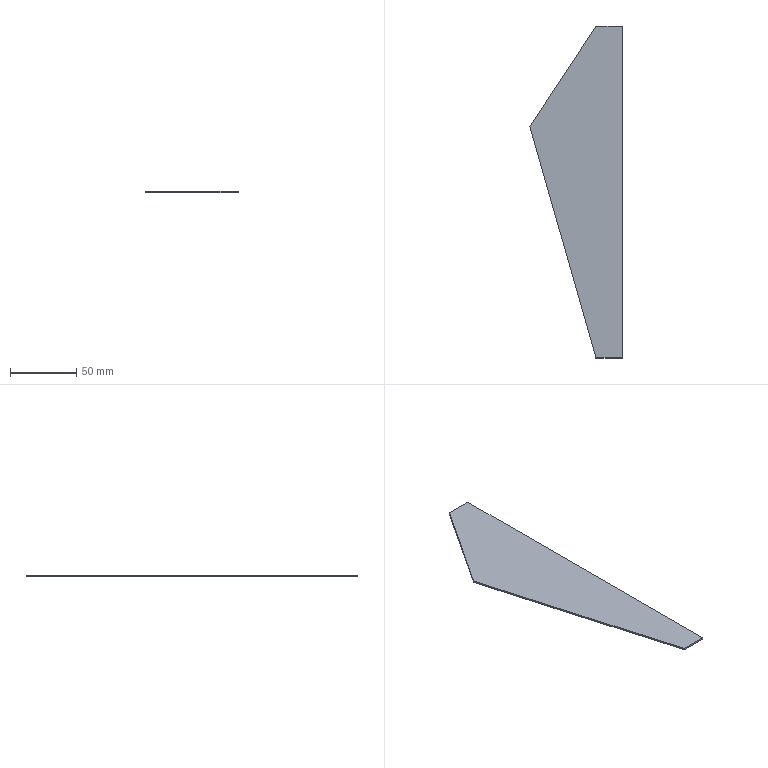Part | SolidWorks | features FlatPattern 1, SMBaseFlange 1, SheetMetal 1 | 1 solid | 7 faces | box 69.783 x 250.8 x 1.2 mm | volume 13490 mm3 | plane 7
STEP:
#1=CARTESIAN_POINT('',(-61.583,173.767,0.));
#2=VERTEX_POINT('',#1);
#3=CARTESIAN_POINT('',(-11.649,-1.,0.));
#4=VERTEX_POINT('',#3);
#5=CARTESIAN_POINT('',(-61.583,173.767,0.));
#6=DIRECTION('',(0.2747,-0.9615,0.));
#7=VECTOR('',#6,1000.);
#8=LINE('',#5,#7);
#9=EDGE_CURVE('',#2,#4,#8,.T.);
#10=ORIENTED_EDGE('',*,*,#9,.F.);
#11=CARTESIAN_POINT('',(-61.583,173.767,-1.2));
#12=VERTEX_POINT('',#11);
#13=CARTESIAN_POINT('',(-61.583,173.767,-1.2));
#14=DIRECTION('',(0.,0.,1.));
#15=VECTOR('',#14,1000.);
#16=LINE('',#13,#15);
#17=EDGE_CURVE('',#12,#2,#16,.T.);
#18=ORIENTED_EDGE('',*,*,#17,.F.);
#19=CARTESIAN_POINT('',(-11.649,-1.,-1.2));
#20=VERTEX_POINT('',#19);
#21=CARTESIAN_POINT('',(-61.583,173.767,-1.2));
#22=DIRECTION('',(0.2747,-0.9615,0.));
#23=VECTOR('',#22,1000.);
#24=LINE('',#21,#23);
#25=EDGE_CURVE('',#12,#20,#24,.T.);
#26=ORIENTED_EDGE('',*,*,#25,.T.);
#27=CARTESIAN_POINT('',(-11.649,-1.,-1.2));
#28=DIRECTION('',(0.,0.,1.));
#29=VECTOR('',#28,1000.);
#30=LINE('',#27,#29);
#31=EDGE_CURVE('',#20,#4,#30,.T.);
#32=ORIENTED_EDGE('',*,*,#31,.T.);
#33=EDGE_LOOP('',(#10,#18,#26,#32));
#34=FACE_OUTER_BOUND('',#33,.T.);
#35=CARTESIAN_POINT('',(-61.583,173.767,-1.2));
#36=DIRECTION('',(-0.9615,-0.2747,0.));
#37=DIRECTION('',(0.2747,-0.9615,0.));
#38=AXIS2_PLACEMENT_3D('',#35,#36,#37);
#39=PLANE('',#38);
#40=ADVANCED_FACE('',(#34),#39,.T.);
#41=CARTESIAN_POINT('',(-11.692,249.8,0.));
#42=VERTEX_POINT('',#41);
#43=CARTESIAN_POINT('',(-61.583,173.767,0.));
#44=DIRECTION('',(-0.5486,-0.8361,0.));
#45=VECTOR('',#44,1000.);
#46=LINE('',#43,#45);
#47=EDGE_CURVE('',#42,#2,#46,.T.);
#48=ORIENTED_EDGE('',*,*,#47,.F.);
#49=CARTESIAN_POINT('',(-11.692,249.8,-1.2));
#50=VERTEX_POINT('',#49);
#51=CARTESIAN_POINT('',(-11.692,249.8,-1.2));
#52=DIRECTION('',(0.,0.,1.));
#53=VECTOR('',#52,1000.);
#54=LINE('',#51,#53);
#55=EDGE_CURVE('',#50,#42,#54,.T.);
#56=ORIENTED_EDGE('',*,*,#55,.F.);
#57=CARTESIAN_POINT('',(-61.583,173.767,-1.2));
#58=DIRECTION('',(-0.5486,-0.8361,0.));
#59=VECTOR('',#58,1000.);
#60=LINE('',#57,#59);
#61=EDGE_CURVE('',#50,#12,#60,.T.);
#62=ORIENTED_EDGE('',*,*,#61,.T.);
#63=ORIENTED_EDGE('',*,*,#17,.T.);
#64=EDGE_LOOP('',(#48,#56,#62,#63));
#65=FACE_OUTER_BOUND('',#64,.T.);
#66=CARTESIAN_POINT('',(-61.583,173.767,-1.2));
#67=DIRECTION('',(-0.8361,0.5486,0.));
#68=DIRECTION('',(-0.5486,-0.8361,0.));
#69=AXIS2_PLACEMENT_3D('',#66,#67,#68);
#70=PLANE('',#69);
#71=ADVANCED_FACE('',(#65),#70,.T.);
#72=CARTESIAN_POINT('',(8.2,249.8,0.));
#73=VERTEX_POINT('',#72);
#74=CARTESIAN_POINT('',(-11.692,249.8,0.));
#75=DIRECTION('',(-1.,0.,0.));
#76=VECTOR('',#75,1000.);
#77=LINE('',#74,#76);
#78=EDGE_CURVE('',#73,#42,#77,.T.);
#79=ORIENTED_EDGE('',*,*,#78,.F.);
#80=CARTESIAN_POINT('',(8.2,249.8,-1.2));
#81=VERTEX_POINT('',#80);
#82=CARTESIAN_POINT('',(8.2,249.8,-1.2));
#83=DIRECTION('',(0.,0.,1.));
#84=VECTOR('',#83,1000.);
#85=LINE('',#82,#84);
#86=EDGE_CURVE('',#81,#73,#85,.T.);
#87=ORIENTED_EDGE('',*,*,#86,.F.);
#88=CARTESIAN_POINT('',(-11.692,249.8,-1.2));
#89=DIRECTION('',(-1.,0.,0.));
#90=VECTOR('',#89,1000.);
#91=LINE('',#88,#90);
#92=EDGE_CURVE('',#81,#50,#91,.T.);
#93=ORIENTED_EDGE('',*,*,#92,.T.);
#94=ORIENTED_EDGE('',*,*,#55,.T.);
#95=EDGE_LOOP('',(#79,#87,#93,#94));
#96=FACE_OUTER_BOUND('',#95,.T.);
#97=CARTESIAN_POINT('',(-11.692,249.8,-1.2));
#98=DIRECTION('',(0.,1.,0.));
#99=DIRECTION('',(0.,0.,1.));
#100=AXIS2_PLACEMENT_3D('',#97,#98,#99);
#101=PLANE('',#100);
#102=ADVANCED_FACE('',(#96),#101,.T.);
#103=CARTESIAN_POINT('',(8.2,-1.,0.));
#104=VERTEX_POINT('',#103);
#105=CARTESIAN_POINT('',(8.2,249.8,0.));
#106=DIRECTION('',(0.,1.,0.));
#107=VECTOR('',#106,1000.);
#108=LINE('',#105,#107);
#109=EDGE_CURVE('',#104,#73,#108,.T.);
#110=ORIENTED_EDGE('',*,*,#109,.F.);
#111=CARTESIAN_POINT('',(8.2,-1.,-1.2));
#112=VERTEX_POINT('',#111);
#113=CARTESIAN_POINT('',(8.2,-1.,-1.2));
#114=DIRECTION('',(0.,0.,1.));
#115=VECTOR('',#114,1000.);
#116=LINE('',#113,#115);
#117=EDGE_CURVE('',#112,#104,#116,.T.);
#118=ORIENTED_EDGE('',*,*,#117,.F.);
#119=CARTESIAN_POINT('',(8.2,249.8,-1.2));
#120=DIRECTION('',(0.,1.,0.));
#121=VECTOR('',#120,1000.);
#122=LINE('',#119,#121);
#123=EDGE_CURVE('',#112,#81,#122,.T.);
#124=ORIENTED_EDGE('',*,*,#123,.T.);
#125=ORIENTED_EDGE('',*,*,#86,.T.);
#126=EDGE_LOOP('',(#110,#118,#124,#125));
#127=FACE_OUTER_BOUND('',#126,.T.);
#128=CARTESIAN_POINT('',(8.2,249.8,-1.2));
#129=DIRECTION('',(1.,0.,0.));
#130=DIRECTION('',(0.,0.,-1.));
#131=AXIS2_PLACEMENT_3D('',#128,#129,#130);
#132=PLANE('',#131);
#133=ADVANCED_FACE('',(#127),#132,.T.);
#134=CARTESIAN_POINT('',(-11.649,-1.,0.));
#135=DIRECTION('',(1.,0.,0.));
#136=VECTOR('',#135,1000.);
#137=LINE('',#134,#136);
#138=EDGE_CURVE('',#4,#104,#137,.T.);
#139=ORIENTED_EDGE('',*,*,#138,.F.);
#140=ORIENTED_EDGE('',*,*,#31,.F.);
#141=CARTESIAN_POINT('',(-11.649,-1.,-1.2));
#142=DIRECTION('',(1.,0.,0.));
#143=VECTOR('',#142,1000.);
#144=LINE('',#141,#143);
#145=EDGE_CURVE('',#20,#112,#144,.T.);
#146=ORIENTED_EDGE('',*,*,#145,.T.);
#147=ORIENTED_EDGE('',*,*,#117,.T.);
#148=EDGE_LOOP('',(#139,#140,#146,#147));
#149=FACE_OUTER_BOUND('',#148,.T.);
#150=CARTESIAN_POINT('',(-11.649,-1.,-1.2));
#151=DIRECTION('',(0.,-1.,0.));
#152=DIRECTION('',(0.,0.,-1.));
#153=AXIS2_PLACEMENT_3D('',#150,#151,#152);
#154=PLANE('',#153);
#155=ADVANCED_FACE('',(#149),#154,.T.);
#156=ORIENTED_EDGE('',*,*,#25,.F.);
#157=ORIENTED_EDGE('',*,*,#61,.F.);
#158=ORIENTED_EDGE('',*,*,#92,.F.);
#159=ORIENTED_EDGE('',*,*,#123,.F.);
#160=ORIENTED_EDGE('',*,*,#145,.F.);
#161=EDGE_LOOP('',(#156,#157,#158,#159,#160));
#162=FACE_OUTER_BOUND('',#161,.T.);
#163=CARTESIAN_POINT('',(-11.649,-1.,-1.2));
#164=DIRECTION('',(0.,0.,1.));
#165=DIRECTION('',(1.,0.,0.));
#166=AXIS2_PLACEMENT_3D('',#163,#164,#165);
#167=PLANE('',#166);
#168=ADVANCED_FACE('',(#162),#167,.F.);
#169=ORIENTED_EDGE('',*,*,#9,.T.);
#170=ORIENTED_EDGE('',*,*,#138,.T.);
#171=ORIENTED_EDGE('',*,*,#109,.T.);
#172=ORIENTED_EDGE('',*,*,#78,.T.);
#173=ORIENTED_EDGE('',*,*,#47,.T.);
#174=EDGE_LOOP('',(#169,#170,#171,#172,#173));
#175=FACE_OUTER_BOUND('',#174,.T.);
#176=CARTESIAN_POINT('',(-11.649,-1.,0.));
#177=DIRECTION('',(0.,0.,1.));
#178=DIRECTION('',(1.,0.,0.));
#179=AXIS2_PLACEMENT_3D('',#176,#177,#178);
#180=PLANE('',#179);
#181=ADVANCED_FACE('',(#175),#180,.T.);
#182=CLOSED_SHELL('',(#40,#71,#102,#133,#155,#168,#181));
#183=MANIFOLD_SOLID_BREP('',#182);
#184=CARTESIAN_POINT('',(0.,0.,0.));
#185=DIRECTION('',(0.,0.,1.));
#186=DIRECTION('',(1.,0.,0.));
#187=AXIS2_PLACEMENT_3D('',#184,#185,#186);
#188=(LENGTH_UNIT()NAMED_UNIT(*)SI_UNIT(.MILLI.,.METRE.));
#189=UNCERTAINTY_MEASURE_WITH_UNIT(LENGTH_MEASURE(0.00001),#188,'','');
#190=(NAMED_UNIT(*)PLANE_ANGLE_UNIT()SI_UNIT($,.RADIAN.));
#191=(NAMED_UNIT(*)SI_UNIT($,.STERADIAN.)SOLID_ANGLE_UNIT());
#192=(GEOMETRIC_REPRESENTATION_CONTEXT(3)GLOBAL_UNCERTAINTY_ASSIGNED_CONTEXT((#189))GLOBAL_UNIT_ASSIGNED_CONTEXT((#188,#190,#191))REPRESENTATION_CONTEXT('',''));
#193=ADVANCED_BREP_SHAPE_REPRESENTATION('',(#183,#187),#192);